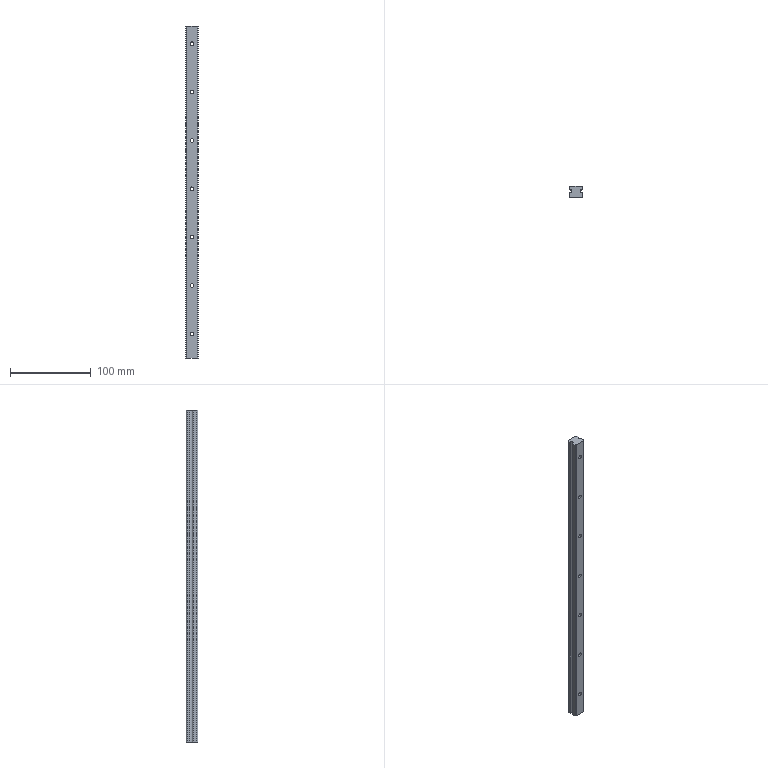Part | Creo | features CUT 8, CURVE 3, DATUM PLANE 3, COORDINATE SYSTEM 1, PATTERN 1, PROTRUSION 1 | 1 solid | 49 faces | box 14.99 x 14 x 412 mm | volume 76604 mm3 | cylinder 30 | plane 19 | commonest cylinder face diameters 4.5 x14 7.5 x14 4.48 x2
STEP:
#1=CARTESIAN_POINT('',(0.,0.,0.));
#2=DIRECTION('',(0.,0.,1.));
#3=DIRECTION('',(1.,0.,0.));
#4=AXIS2_PLACEMENT_3D('',#1,#2,#3);
#5=CARTESIAN_POINT('',(-7.49,0.995,-206.));
#6=VERTEX_POINT('',#5);
#7=CARTESIAN_POINT('',(-6.495,0.,-206.));
#8=VERTEX_POINT('',#7);
#9=CARTESIAN_POINT('',(-7.49,0.995,-206.));
#10=DIRECTION('',(0.7071,-0.7071,0.));
#11=VECTOR('',#10,1.407);
#12=LINE('',#9,#11);
#13=EDGE_CURVE('',#6,#8,#12,.T.);
#14=ORIENTED_EDGE('',*,*,#13,.T.);
#15=CARTESIAN_POINT('',(6.505,0.,-206.));
#16=VERTEX_POINT('',#15);
#17=CARTESIAN_POINT('',(-6.495,0.,-206.));
#18=DIRECTION('',(1.,0.,0.));
#19=VECTOR('',#18,13.);
#20=LINE('',#17,#19);
#21=EDGE_CURVE('',#8,#16,#20,.T.);
#22=ORIENTED_EDGE('',*,*,#21,.T.);
#23=CARTESIAN_POINT('',(7.5,0.995,-206.));
#24=VERTEX_POINT('',#23);
#25=CARTESIAN_POINT('',(6.505,0.,-206.));
#26=DIRECTION('',(0.7071,0.7071,0.));
#27=VECTOR('',#26,1.407);
#28=LINE('',#25,#27);
#29=EDGE_CURVE('',#16,#24,#28,.T.);
#30=ORIENTED_EDGE('',*,*,#29,.T.);
#31=CARTESIAN_POINT('',(7.5,5.525,-206.));
#32=VERTEX_POINT('',#31);
#33=CARTESIAN_POINT('',(7.5,0.995,-206.));
#34=DIRECTION('',(0.,1.,0.));
#35=VECTOR('',#34,4.53);
#36=LINE('',#33,#35);
#37=EDGE_CURVE('',#24,#32,#36,.T.);
#38=ORIENTED_EDGE('',*,*,#37,.T.);
#39=CARTESIAN_POINT('',(7.5,10.005,-206.));
#40=VERTEX_POINT('',#39);
#41=CARTESIAN_POINT('',(7.5,7.765,-206.));
#42=DIRECTION('',(0.,0.,-1.));
#43=DIRECTION('',(0.,-1.,0.));
#44=AXIS2_PLACEMENT_3D('',#41,#42,#43);
#45=CIRCLE('',#44,2.24);
#46=EDGE_CURVE('',#32,#40,#45,.T.);
#47=ORIENTED_EDGE('',*,*,#46,.T.);
#48=CARTESIAN_POINT('',(7.5,13.005,-206.));
#49=VERTEX_POINT('',#48);
#50=CARTESIAN_POINT('',(7.5,10.005,-206.));
#51=DIRECTION('',(0.,1.,0.));
#52=VECTOR('',#51,3.);
#53=LINE('',#50,#52);
#54=EDGE_CURVE('',#40,#49,#53,.T.);
#55=ORIENTED_EDGE('',*,*,#54,.T.);
#56=CARTESIAN_POINT('',(6.505,14.,-206.));
#57=VERTEX_POINT('',#56);
#58=CARTESIAN_POINT('',(7.5,13.005,-206.));
#59=DIRECTION('',(-0.7071,0.7071,0.));
#60=VECTOR('',#59,1.407);
#61=LINE('',#58,#60);
#62=EDGE_CURVE('',#49,#57,#61,.T.);
#63=ORIENTED_EDGE('',*,*,#62,.T.);
#64=CARTESIAN_POINT('',(-6.495,14.,-206.));
#65=VERTEX_POINT('',#64);
#66=CARTESIAN_POINT('',(6.505,14.,-206.));
#67=DIRECTION('',(-1.,0.,0.));
#68=VECTOR('',#67,13.);
#69=LINE('',#66,#68);
#70=EDGE_CURVE('',#57,#65,#69,.T.);
#71=ORIENTED_EDGE('',*,*,#70,.T.);
#72=CARTESIAN_POINT('',(-7.49,13.005,-206.));
#73=VERTEX_POINT('',#72);
#74=CARTESIAN_POINT('',(-6.495,14.,-206.));
#75=DIRECTION('',(-0.7071,-0.7071,0.));
#76=VECTOR('',#75,1.407);
#77=LINE('',#74,#76);
#78=EDGE_CURVE('',#65,#73,#77,.T.);
#79=ORIENTED_EDGE('',*,*,#78,.T.);
#80=CARTESIAN_POINT('',(-7.49,10.005,-206.));
#81=VERTEX_POINT('',#80);
#82=CARTESIAN_POINT('',(-7.49,13.005,-206.));
#83=DIRECTION('',(0.,-1.,0.));
#84=VECTOR('',#83,3.);
#85=LINE('',#82,#84);
#86=EDGE_CURVE('',#73,#81,#85,.T.);
#87=ORIENTED_EDGE('',*,*,#86,.T.);
#88=CARTESIAN_POINT('',(-7.49,5.525,-206.));
#89=VERTEX_POINT('',#88);
#90=CARTESIAN_POINT('',(-7.49,7.765,-206.));
#91=DIRECTION('',(0.,0.,-1.));
#92=DIRECTION('',(0.,1.,0.));
#93=AXIS2_PLACEMENT_3D('',#90,#91,#92);
#94=CIRCLE('',#93,2.24);
#95=EDGE_CURVE('',#81,#89,#94,.T.);
#96=ORIENTED_EDGE('',*,*,#95,.T.);
#97=CARTESIAN_POINT('',(-7.49,5.525,-206.));
#98=DIRECTION('',(0.,-1.,0.));
#99=VECTOR('',#98,4.53);
#100=LINE('',#97,#99);
#101=EDGE_CURVE('',#89,#6,#100,.T.);
#102=ORIENTED_EDGE('',*,*,#101,.T.);
#103=EDGE_LOOP('',(#14,#22,#30,#38,#47,#55,#63,#71,#79,#87,#96,#102));
#104=FACE_OUTER_BOUND('',#103,.F.);
#105=CARTESIAN_POINT('',(0.,0.,-206.));
#106=DIRECTION('',(0.,0.,1.));
#107=DIRECTION('',(1.,0.,0.));
#108=AXIS2_PLACEMENT_3D('',#105,#106,#107);
#109=PLANE('',#108);
#110=ADVANCED_FACE('',(#104),#109,.F.);
#111=ORIENTED_EDGE('',*,*,#13,.F.);
#112=CARTESIAN_POINT('',(-7.49,0.995,206.));
#113=VERTEX_POINT('',#112);
#114=CARTESIAN_POINT('',(-7.49,0.995,-206.));
#115=DIRECTION('',(0.,0.,1.));
#116=VECTOR('',#115,412.);
#117=LINE('',#114,#116);
#118=EDGE_CURVE('',#6,#113,#117,.T.);
#119=ORIENTED_EDGE('',*,*,#118,.T.);
#120=CARTESIAN_POINT('',(-6.495,0.,206.));
#121=VERTEX_POINT('',#120);
#122=CARTESIAN_POINT('',(-7.49,0.995,206.));
#123=DIRECTION('',(0.7071,-0.7071,0.));
#124=VECTOR('',#123,1.407);
#125=LINE('',#122,#124);
#126=EDGE_CURVE('',#113,#121,#125,.T.);
#127=ORIENTED_EDGE('',*,*,#126,.T.);
#128=CARTESIAN_POINT('',(-6.495,0.,-206.));
#129=DIRECTION('',(0.,0.,1.));
#130=VECTOR('',#129,412.);
#131=LINE('',#128,#130);
#132=EDGE_CURVE('',#8,#121,#131,.T.);
#133=ORIENTED_EDGE('',*,*,#132,.F.);
#134=EDGE_LOOP('',(#111,#119,#127,#133));
#135=FACE_OUTER_BOUND('',#134,.F.);
#136=CARTESIAN_POINT('',(-7.49,0.995,-206.));
#137=DIRECTION('',(-0.7071,-0.7071,0.));
#138=DIRECTION('',(0.7071,-0.7071,0.));
#139=AXIS2_PLACEMENT_3D('',#136,#137,#138);
#140=PLANE('',#139);
#141=ADVANCED_FACE('',(#135),#140,.T.);
#142=ORIENTED_EDGE('',*,*,#101,.F.);
#143=CARTESIAN_POINT('',(-7.49,5.525,206.));
#144=VERTEX_POINT('',#143);
#145=CARTESIAN_POINT('',(-7.49,5.525,-206.));
#146=DIRECTION('',(0.,0.,1.));
#147=VECTOR('',#146,412.);
#148=LINE('',#145,#147);
#149=EDGE_CURVE('',#89,#144,#148,.T.);
#150=ORIENTED_EDGE('',*,*,#149,.T.);
#151=CARTESIAN_POINT('',(-7.49,5.525,206.));
#152=DIRECTION('',(0.,-1.,0.));
#153=VECTOR('',#152,4.53);
#154=LINE('',#151,#153);
#155=EDGE_CURVE('',#144,#113,#154,.T.);
#156=ORIENTED_EDGE('',*,*,#155,.T.);
#157=ORIENTED_EDGE('',*,*,#118,.F.);
#158=EDGE_LOOP('',(#142,#150,#156,#157));
#159=FACE_OUTER_BOUND('',#158,.F.);
#160=CARTESIAN_POINT('',(-7.49,5.525,-206.));
#161=DIRECTION('',(-1.,0.,0.));
#162=DIRECTION('',(0.,-1.,0.));
#163=AXIS2_PLACEMENT_3D('',#160,#161,#162);
#164=PLANE('',#163);
#165=ADVANCED_FACE('',(#159),#164,.T.);
#166=ORIENTED_EDGE('',*,*,#95,.F.);
#167=CARTESIAN_POINT('',(-7.49,10.005,206.));
#168=VERTEX_POINT('',#167);
#169=CARTESIAN_POINT('',(-7.49,10.005,-206.));
#170=DIRECTION('',(0.,0.,1.));
#171=VECTOR('',#170,412.);
#172=LINE('',#169,#171);
#173=EDGE_CURVE('',#81,#168,#172,.T.);
#174=ORIENTED_EDGE('',*,*,#173,.T.);
#175=CARTESIAN_POINT('',(-7.49,7.765,206.));
#176=DIRECTION('',(0.,0.,-1.));
#177=DIRECTION('',(0.,1.,0.));
#178=AXIS2_PLACEMENT_3D('',#175,#176,#177);
#179=CIRCLE('',#178,2.24);
#180=EDGE_CURVE('',#168,#144,#179,.T.);
#181=ORIENTED_EDGE('',*,*,#180,.T.);
#182=ORIENTED_EDGE('',*,*,#149,.F.);
#183=EDGE_LOOP('',(#166,#174,#181,#182));
#184=FACE_OUTER_BOUND('',#183,.F.);
#185=CARTESIAN_POINT('',(-7.49,7.765,-206.));
#186=DIRECTION('',(0.,0.,1.));
#187=DIRECTION('',(1.,0.,0.));
#188=AXIS2_PLACEMENT_3D('',#185,#186,#187);
#189=CYLINDRICAL_SURFACE('',#188,2.24);
#190=ADVANCED_FACE('',(#184),#189,.F.);
#191=ORIENTED_EDGE('',*,*,#86,.F.);
#192=CARTESIAN_POINT('',(-7.49,13.005,206.));
#193=VERTEX_POINT('',#192);
#194=CARTESIAN_POINT('',(-7.49,13.005,-206.));
#195=DIRECTION('',(0.,0.,1.));
#196=VECTOR('',#195,412.);
#197=LINE('',#194,#196);
#198=EDGE_CURVE('',#73,#193,#197,.T.);
#199=ORIENTED_EDGE('',*,*,#198,.T.);
#200=CARTESIAN_POINT('',(-7.49,13.005,206.));
#201=DIRECTION('',(0.,-1.,0.));
#202=VECTOR('',#201,3.);
#203=LINE('',#200,#202);
#204=EDGE_CURVE('',#193,#168,#203,.T.);
#205=ORIENTED_EDGE('',*,*,#204,.T.);
#206=ORIENTED_EDGE('',*,*,#173,.F.);
#207=EDGE_LOOP('',(#191,#199,#205,#206));
#208=FACE_OUTER_BOUND('',#207,.F.);
#209=CARTESIAN_POINT('',(-7.49,13.005,-206.));
#210=DIRECTION('',(-1.,0.,0.));
#211=DIRECTION('',(0.,-1.,0.));
#212=AXIS2_PLACEMENT_3D('',#209,#210,#211);
#213=PLANE('',#212);
#214=ADVANCED_FACE('',(#208),#213,.T.);
#215=ORIENTED_EDGE('',*,*,#78,.F.);
#216=CARTESIAN_POINT('',(-6.495,14.,206.));
#217=VERTEX_POINT('',#216);
#218=CARTESIAN_POINT('',(-6.495,14.,-206.));
#219=DIRECTION('',(0.,0.,1.));
#220=VECTOR('',#219,412.);
#221=LINE('',#218,#220);
#222=EDGE_CURVE('',#65,#217,#221,.T.);
#223=ORIENTED_EDGE('',*,*,#222,.T.);
#224=CARTESIAN_POINT('',(-6.495,14.,206.));
#225=DIRECTION('',(-0.7071,-0.7071,0.));
#226=VECTOR('',#225,1.407);
#227=LINE('',#224,#226);
#228=EDGE_CURVE('',#217,#193,#227,.T.);
#229=ORIENTED_EDGE('',*,*,#228,.T.);
#230=ORIENTED_EDGE('',*,*,#198,.F.);
#231=EDGE_LOOP('',(#215,#223,#229,#230));
#232=FACE_OUTER_BOUND('',#231,.F.);
#233=CARTESIAN_POINT('',(-6.495,14.,-206.));
#234=DIRECTION('',(-0.7071,0.7071,0.));
#235=DIRECTION('',(-0.7071,-0.7071,0.));
#236=AXIS2_PLACEMENT_3D('',#233,#234,#235);
#237=PLANE('',#236);
#238=ADVANCED_FACE('',(#232),#237,.T.);
#239=ORIENTED_EDGE('',*,*,#70,.F.);
#240=CARTESIAN_POINT('',(6.505,14.,206.));
#241=VERTEX_POINT('',#240);
#242=CARTESIAN_POINT('',(6.505,14.,-206.));
#243=DIRECTION('',(0.,0.,1.));
#244=VECTOR('',#243,412.);
#245=LINE('',#242,#244);
#246=EDGE_CURVE('',#57,#241,#245,.T.);
#247=ORIENTED_EDGE('',*,*,#246,.T.);
#248=CARTESIAN_POINT('',(6.505,14.,206.));
#249=DIRECTION('',(-1.,0.,0.));
#250=VECTOR('',#249,13.);
#251=LINE('',#248,#250);
#252=EDGE_CURVE('',#241,#217,#251,.T.);
#253=ORIENTED_EDGE('',*,*,#252,.T.);
#254=ORIENTED_EDGE('',*,*,#222,.F.);
#255=EDGE_LOOP('',(#239,#247,#253,#254));
#256=FACE_OUTER_BOUND('',#255,.F.);
#257=CARTESIAN_POINT('',(0.,14.,-172.25));
#258=VERTEX_POINT('',#257);
#259=CARTESIAN_POINT('',(0.,14.,-179.75));
#260=VERTEX_POINT('',#259);
#261=CARTESIAN_POINT('',(0.,14.,-176.));
#262=DIRECTION('',(0.,1.,0.));
#263=DIRECTION('',(0.,0.,1.));
#264=AXIS2_PLACEMENT_3D('',#261,#262,#263);
#265=CIRCLE('',#264,3.75);
#266=EDGE_CURVE('',#258,#260,#265,.T.);
#267=ORIENTED_EDGE('',*,*,#266,.T.);
#268=CARTESIAN_POINT('',(0.,14.,-176.));
#269=DIRECTION('',(0.,1.,0.));
#270=DIRECTION('',(0.,0.,-1.));
#271=AXIS2_PLACEMENT_3D('',#268,#269,#270);
#272=CIRCLE('',#271,3.75);
#273=EDGE_CURVE('',#260,#258,#272,.T.);
#274=ORIENTED_EDGE('',*,*,#273,.T.);
#275=EDGE_LOOP('',(#267,#274));
#276=FACE_BOUND('',#275,.F.);
#277=CARTESIAN_POINT('',(0.,14.,-112.25));
#278=VERTEX_POINT('',#277);
#279=CARTESIAN_POINT('',(0.,14.,-119.75));
#280=VERTEX_POINT('',#279);
#281=CARTESIAN_POINT('',(0.,14.,-116.));
#282=DIRECTION('',(0.,1.,0.));
#283=DIRECTION('',(0.,0.,1.));
#284=AXIS2_PLACEMENT_3D('',#281,#282,#283);
#285=CIRCLE('',#284,3.75);
#286=EDGE_CURVE('',#278,#280,#285,.T.);
#287=ORIENTED_EDGE('',*,*,#286,.T.);
#288=CARTESIAN_POINT('',(0.,14.,-116.));
#289=DIRECTION('',(0.,1.,0.));
#290=DIRECTION('',(0.,0.,-1.));
#291=AXIS2_PLACEMENT_3D('',#288,#289,#290);
#292=CIRCLE('',#291,3.75);
#293=EDGE_CURVE('',#280,#278,#292,.T.);
#294=ORIENTED_EDGE('',*,*,#293,.T.);
#295=EDGE_LOOP('',(#287,#294));
#296=FACE_BOUND('',#295,.F.);
#297=CARTESIAN_POINT('',(0.,14.,-52.25));
#298=VERTEX_POINT('',#297);
#299=CARTESIAN_POINT('',(0.,14.,-59.75));
#300=VERTEX_POINT('',#299);
#301=CARTESIAN_POINT('',(0.,14.,-56.));
#302=DIRECTION('',(0.,1.,0.));
#303=DIRECTION('',(0.,0.,1.));
#304=AXIS2_PLACEMENT_3D('',#301,#302,#303);
#305=CIRCLE('',#304,3.75);
#306=EDGE_CURVE('',#298,#300,#305,.T.);
#307=ORIENTED_EDGE('',*,*,#306,.T.);
#308=CARTESIAN_POINT('',(0.,14.,-56.));
#309=DIRECTION('',(0.,1.,0.));
#310=DIRECTION('',(0.,0.,-1.));
#311=AXIS2_PLACEMENT_3D('',#308,#309,#310);
#312=CIRCLE('',#311,3.75);
#313=EDGE_CURVE('',#300,#298,#312,.T.);
#314=ORIENTED_EDGE('',*,*,#313,.T.);
#315=EDGE_LOOP('',(#307,#314));
#316=FACE_BOUND('',#315,.F.);
#317=CARTESIAN_POINT('',(0.,14.,7.75));
#318=VERTEX_POINT('',#317);
#319=CARTESIAN_POINT('',(0.,14.,0.25));
#320=VERTEX_POINT('',#319);
#321=CARTESIAN_POINT('',(0.,14.,4.));
#322=DIRECTION('',(0.,1.,0.));
#323=DIRECTION('',(0.,0.,1.));
#324=AXIS2_PLACEMENT_3D('',#321,#322,#323);
#325=CIRCLE('',#324,3.75);
#326=EDGE_CURVE('',#318,#320,#325,.T.);
#327=ORIENTED_EDGE('',*,*,#326,.T.);
#328=CARTESIAN_POINT('',(0.,14.,4.));
#329=DIRECTION('',(0.,1.,0.));
#330=DIRECTION('',(0.,0.,-1.));
#331=AXIS2_PLACEMENT_3D('',#328,#329,#330);
#332=CIRCLE('',#331,3.75);
#333=EDGE_CURVE('',#320,#318,#332,.T.);
#334=ORIENTED_EDGE('',*,*,#333,.T.);
#335=EDGE_LOOP('',(#327,#334));
#336=FACE_BOUND('',#335,.F.);
#337=CARTESIAN_POINT('',(0.,14.,67.75));
#338=VERTEX_POINT('',#337);
#339=CARTESIAN_POINT('',(0.,14.,60.25));
#340=VERTEX_POINT('',#339);
#341=CARTESIAN_POINT('',(0.,14.,64.));
#342=DIRECTION('',(0.,1.,0.));
#343=DIRECTION('',(0.,0.,1.));
#344=AXIS2_PLACEMENT_3D('',#341,#342,#343);
#345=CIRCLE('',#344,3.75);
#346=EDGE_CURVE('',#338,#340,#345,.T.);
#347=ORIENTED_EDGE('',*,*,#346,.T.);
#348=CARTESIAN_POINT('',(0.,14.,64.));
#349=DIRECTION('',(0.,1.,0.));
#350=DIRECTION('',(0.,0.,-1.));
#351=AXIS2_PLACEMENT_3D('',#348,#349,#350);
#352=CIRCLE('',#351,3.75);
#353=EDGE_CURVE('',#340,#338,#352,.T.);
#354=ORIENTED_EDGE('',*,*,#353,.T.);
#355=EDGE_LOOP('',(#347,#354));
#356=FACE_BOUND('',#355,.F.);
#357=CARTESIAN_POINT('',(0.,14.,127.75));
#358=VERTEX_POINT('',#357);
#359=CARTESIAN_POINT('',(0.,14.,120.25));
#360=VERTEX_POINT('',#359);
#361=CARTESIAN_POINT('',(0.,14.,124.));
#362=DIRECTION('',(0.,1.,0.));
#363=DIRECTION('',(0.,0.,1.));
#364=AXIS2_PLACEMENT_3D('',#361,#362,#363);
#365=CIRCLE('',#364,3.75);
#366=EDGE_CURVE('',#358,#360,#365,.T.);
#367=ORIENTED_EDGE('',*,*,#366,.T.);
#368=CARTESIAN_POINT('',(0.,14.,124.));
#369=DIRECTION('',(0.,1.,0.));
#370=DIRECTION('',(0.,0.,-1.));
#371=AXIS2_PLACEMENT_3D('',#368,#369,#370);
#372=CIRCLE('',#371,3.75);
#373=EDGE_CURVE('',#360,#358,#372,.T.);
#374=ORIENTED_EDGE('',*,*,#373,.T.);
#375=EDGE_LOOP('',(#367,#374));
#376=FACE_BOUND('',#375,.F.);
#377=CARTESIAN_POINT('',(0.,14.,187.75));
#378=VERTEX_POINT('',#377);
#379=CARTESIAN_POINT('',(0.,14.,180.25));
#380=VERTEX_POINT('',#379);
#381=CARTESIAN_POINT('',(0.,14.,184.));
#382=DIRECTION('',(0.,1.,0.));
#383=DIRECTION('',(0.,0.,1.));
#384=AXIS2_PLACEMENT_3D('',#381,#382,#383);
#385=CIRCLE('',#384,3.75);
#386=EDGE_CURVE('',#378,#380,#385,.T.);
#387=ORIENTED_EDGE('',*,*,#386,.T.);
#388=CARTESIAN_POINT('',(0.,14.,184.));
#389=DIRECTION('',(0.,1.,0.));
#390=DIRECTION('',(0.,0.,-1.));
#391=AXIS2_PLACEMENT_3D('',#388,#389,#390);
#392=CIRCLE('',#391,3.75);
#393=EDGE_CURVE('',#380,#378,#392,.T.);
#394=ORIENTED_EDGE('',*,*,#393,.T.);
#395=EDGE_LOOP('',(#387,#394));
#396=FACE_BOUND('',#395,.F.);
#397=CARTESIAN_POINT('',(6.505,14.,-206.));
#398=DIRECTION('',(0.,1.,0.));
#399=DIRECTION('',(-1.,0.,0.));
#400=AXIS2_PLACEMENT_3D('',#397,#398,#399);
#401=PLANE('',#400);
#402=ADVANCED_FACE('',(#256,#276,#296,#316,#336,#356,#376,#396),#401,.T.);
#403=ORIENTED_EDGE('',*,*,#62,.F.);
#404=CARTESIAN_POINT('',(7.5,13.005,206.));
#405=VERTEX_POINT('',#404);
#406=CARTESIAN_POINT('',(7.5,13.005,-206.));
#407=DIRECTION('',(0.,0.,1.));
#408=VECTOR('',#407,412.);
#409=LINE('',#406,#408);
#410=EDGE_CURVE('',#49,#405,#409,.T.);
#411=ORIENTED_EDGE('',*,*,#410,.T.);
#412=CARTESIAN_POINT('',(7.5,13.005,206.));
#413=DIRECTION('',(-0.7071,0.7071,0.));
#414=VECTOR('',#413,1.407);
#415=LINE('',#412,#414);
#416=EDGE_CURVE('',#405,#241,#415,.T.);
#417=ORIENTED_EDGE('',*,*,#416,.T.);
#418=ORIENTED_EDGE('',*,*,#246,.F.);
#419=EDGE_LOOP('',(#403,#411,#417,#418));
#420=FACE_OUTER_BOUND('',#419,.F.);
#421=CARTESIAN_POINT('',(7.5,13.005,-206.));
#422=DIRECTION('',(0.7071,0.7071,0.));
#423=DIRECTION('',(-0.7071,0.7071,0.));
#424=AXIS2_PLACEMENT_3D('',#421,#422,#423);
#425=PLANE('',#424);
#426=ADVANCED_FACE('',(#420),#425,.T.);
#427=ORIENTED_EDGE('',*,*,#54,.F.);
#428=CARTESIAN_POINT('',(7.5,10.005,206.));
#429=VERTEX_POINT('',#428);
#430=CARTESIAN_POINT('',(7.5,10.005,-206.));
#431=DIRECTION('',(0.,0.,1.));
#432=VECTOR('',#431,412.);
#433=LINE('',#430,#432);
#434=EDGE_CURVE('',#40,#429,#433,.T.);
#435=ORIENTED_EDGE('',*,*,#434,.T.);
#436=CARTESIAN_POINT('',(7.5,10.005,206.));
#437=DIRECTION('',(0.,1.,0.));
#438=VECTOR('',#437,3.);
#439=LINE('',#436,#438);
#440=EDGE_CURVE('',#429,#405,#439,.T.);
#441=ORIENTED_EDGE('',*,*,#440,.T.);
#442=ORIENTED_EDGE('',*,*,#410,.F.);
#443=EDGE_LOOP('',(#427,#435,#441,#442));
#444=FACE_OUTER_BOUND('',#443,.F.);
#445=CARTESIAN_POINT('',(7.5,10.005,-206.));
#446=DIRECTION('',(1.,0.,0.));
#447=DIRECTION('',(0.,1.,0.));
#448=AXIS2_PLACEMENT_3D('',#445,#446,#447);
#449=PLANE('',#448);
#450=ADVANCED_FACE('',(#444),#449,.T.);
#451=ORIENTED_EDGE('',*,*,#46,.F.);
#452=CARTESIAN_POINT('',(7.5,5.525,206.));
#453=VERTEX_POINT('',#452);
#454=CARTESIAN_POINT('',(7.5,5.525,-206.));
#455=DIRECTION('',(0.,0.,1.));
#456=VECTOR('',#455,412.);
#457=LINE('',#454,#456);
#458=EDGE_CURVE('',#32,#453,#457,.T.);
#459=ORIENTED_EDGE('',*,*,#458,.T.);
#460=CARTESIAN_POINT('',(7.5,7.765,206.));
#461=DIRECTION('',(0.,0.,-1.));
#462=DIRECTION('',(0.,-1.,0.));
#463=AXIS2_PLACEMENT_3D('',#460,#461,#462);
#464=CIRCLE('',#463,2.24);
#465=EDGE_CURVE('',#453,#429,#464,.T.);
#466=ORIENTED_EDGE('',*,*,#465,.T.);
#467=ORIENTED_EDGE('',*,*,#434,.F.);
#468=EDGE_LOOP('',(#451,#459,#466,#467));
#469=FACE_OUTER_BOUND('',#468,.F.);
#470=CARTESIAN_POINT('',(7.5,7.765,-206.));
#471=DIRECTION('',(0.,0.,1.));
#472=DIRECTION('',(1.,0.,0.));
#473=AXIS2_PLACEMENT_3D('',#470,#471,#472);
#474=CYLINDRICAL_SURFACE('',#473,2.24);
#475=ADVANCED_FACE('',(#469),#474,.F.);
#476=ORIENTED_EDGE('',*,*,#37,.F.);
#477=CARTESIAN_POINT('',(7.5,0.995,206.));
#478=VERTEX_POINT('',#477);
#479=CARTESIAN_POINT('',(7.5,0.995,-206.));
#480=DIRECTION('',(0.,0.,1.));
#481=VECTOR('',#480,412.);
#482=LINE('',#479,#481);
#483=EDGE_CURVE('',#24,#478,#482,.T.);
#484=ORIENTED_EDGE('',*,*,#483,.T.);
#485=CARTESIAN_POINT('',(7.5,0.995,206.));
#486=DIRECTION('',(0.,1.,0.));
#487=VECTOR('',#486,4.53);
#488=LINE('',#485,#487);
#489=EDGE_CURVE('',#478,#453,#488,.T.);
#490=ORIENTED_EDGE('',*,*,#489,.T.);
#491=ORIENTED_EDGE('',*,*,#458,.F.);
#492=EDGE_LOOP('',(#476,#484,#490,#491));
#493=FACE_OUTER_BOUND('',#492,.F.);
#494=CARTESIAN_POINT('',(7.5,0.995,-206.));
#495=DIRECTION('',(1.,0.,0.));
#496=DIRECTION('',(0.,1.,0.));
#497=AXIS2_PLACEMENT_3D('',#494,#495,#496);
#498=PLANE('',#497);
#499=ADVANCED_FACE('',(#493),#498,.T.);
#500=ORIENTED_EDGE('',*,*,#29,.F.);
#501=CARTESIAN_POINT('',(6.505,0.,206.));
#502=VERTEX_POINT('',#501);
#503=CARTESIAN_POINT('',(6.505,0.,-206.));
#504=DIRECTION('',(0.,0.,1.));
#505=VECTOR('',#504,412.);
#506=LINE('',#503,#505);
#507=EDGE_CURVE('',#16,#502,#506,.T.);
#508=ORIENTED_EDGE('',*,*,#507,.T.);
#509=CARTESIAN_POINT('',(6.505,0.,206.));
#510=DIRECTION('',(0.7071,0.7071,0.));
#511=VECTOR('',#510,1.407);
#512=LINE('',#509,#511);
#513=EDGE_CURVE('',#502,#478,#512,.T.);
#514=ORIENTED_EDGE('',*,*,#513,.T.);
#515=ORIENTED_EDGE('',*,*,#483,.F.);
#516=EDGE_LOOP('',(#500,#508,#514,#515));
#517=FACE_OUTER_BOUND('',#516,.F.);
#518=CARTESIAN_POINT('',(6.505,0.,-206.));
#519=DIRECTION('',(0.7071,-0.7071,0.));
#520=DIRECTION('',(0.7071,0.7071,0.));
#521=AXIS2_PLACEMENT_3D('',#518,#519,#520);
#522=PLANE('',#521);
#523=ADVANCED_FACE('',(#517),#522,.T.);
#524=ORIENTED_EDGE('',*,*,#21,.F.);
#525=ORIENTED_EDGE('',*,*,#132,.T.);
#526=CARTESIAN_POINT('',(-6.495,0.,206.));
#527=DIRECTION('',(1.,0.,0.));
#528=VECTOR('',#527,13.);
#529=LINE('',#526,#528);
#530=EDGE_CURVE('',#121,#502,#529,.T.);
#531=ORIENTED_EDGE('',*,*,#530,.T.);
#532=ORIENTED_EDGE('',*,*,#507,.F.);
#533=EDGE_LOOP('',(#524,#525,#531,#532));
#534=FACE_OUTER_BOUND('',#533,.F.);
#535=CARTESIAN_POINT('',(0.,0.,-173.75));
#536=VERTEX_POINT('',#535);
#537=CARTESIAN_POINT('',(0.,0.,-178.25));
#538=VERTEX_POINT('',#537);
#539=CARTESIAN_POINT('',(0.,0.,-176.));
#540=DIRECTION('',(0.,1.,0.));
#541=DIRECTION('',(0.,0.,1.));
#542=AXIS2_PLACEMENT_3D('',#539,#540,#541);
#543=CIRCLE('',#542,2.25);
#544=EDGE_CURVE('',#536,#538,#543,.T.);
#545=ORIENTED_EDGE('',*,*,#544,.F.);
#546=CARTESIAN_POINT('',(0.,0.,-176.));
#547=DIRECTION('',(0.,1.,0.));
#548=DIRECTION('',(0.,0.,-1.));
#549=AXIS2_PLACEMENT_3D('',#546,#547,#548);
#550=CIRCLE('',#549,2.25);
#551=EDGE_CURVE('',#538,#536,#550,.T.);
#552=ORIENTED_EDGE('',*,*,#551,.F.);
#553=EDGE_LOOP('',(#545,#552));
#554=FACE_BOUND('',#553,.F.);
#555=CARTESIAN_POINT('',(0.,0.,-113.75));
#556=VERTEX_POINT('',#555);
#557=CARTESIAN_POINT('',(0.,0.,-118.25));
#558=VERTEX_POINT('',#557);
#559=CARTESIAN_POINT('',(0.,0.,-116.));
#560=DIRECTION('',(0.,1.,0.));
#561=DIRECTION('',(0.,0.,1.));
#562=AXIS2_PLACEMENT_3D('',#559,#560,#561);
#563=CIRCLE('',#562,2.25);
#564=EDGE_CURVE('',#556,#558,#563,.T.);
#565=ORIENTED_EDGE('',*,*,#564,.F.);
#566=CARTESIAN_POINT('',(0.,0.,-116.));
#567=DIRECTION('',(0.,1.,0.));
#568=DIRECTION('',(0.,0.,-1.));
#569=AXIS2_PLACEMENT_3D('',#566,#567,#568);
#570=CIRCLE('',#569,2.25);
#571=EDGE_CURVE('',#558,#556,#570,.T.);
#572=ORIENTED_EDGE('',*,*,#571,.F.);
#573=EDGE_LOOP('',(#565,#572));
#574=FACE_BOUND('',#573,.F.);
#575=CARTESIAN_POINT('',(0.,0.,-53.75));
#576=VERTEX_POINT('',#575);
#577=CARTESIAN_POINT('',(0.,0.,-58.25));
#578=VERTEX_POINT('',#577);
#579=CARTESIAN_POINT('',(0.,0.,-56.));
#580=DIRECTION('',(0.,1.,0.));
#581=DIRECTION('',(0.,0.,1.));
#582=AXIS2_PLACEMENT_3D('',#579,#580,#581);
#583=CIRCLE('',#582,2.25);
#584=EDGE_CURVE('',#576,#578,#583,.T.);
#585=ORIENTED_EDGE('',*,*,#584,.F.);
#586=CARTESIAN_POINT('',(0.,0.,-56.));
#587=DIRECTION('',(0.,1.,0.));
#588=DIRECTION('',(0.,0.,-1.));
#589=AXIS2_PLACEMENT_3D('',#586,#587,#588);
#590=CIRCLE('',#589,2.25);
#591=EDGE_CURVE('',#578,#576,#590,.T.);
#592=ORIENTED_EDGE('',*,*,#591,.F.);
#593=EDGE_LOOP('',(#585,#592));
#594=FACE_BOUND('',#593,.F.);
#595=CARTESIAN_POINT('',(0.,0.,6.25));
#596=VERTEX_POINT('',#595);
#597=CARTESIAN_POINT('',(0.,0.,1.75));
#598=VERTEX_POINT('',#597);
#599=CARTESIAN_POINT('',(0.,0.,4.));
#600=DIRECTION('',(0.,1.,0.));
#601=DIRECTION('',(0.,0.,1.));
#602=AXIS2_PLACEMENT_3D('',#599,#600,#601);
#603=CIRCLE('',#602,2.25);
#604=EDGE_CURVE('',#596,#598,#603,.T.);
#605=ORIENTED_EDGE('',*,*,#604,.F.);
#606=CARTESIAN_POINT('',(0.,0.,4.));
#607=DIRECTION('',(0.,1.,0.));
#608=DIRECTION('',(0.,0.,-1.));
#609=AXIS2_PLACEMENT_3D('',#606,#607,#608);
#610=CIRCLE('',#609,2.25);
#611=EDGE_CURVE('',#598,#596,#610,.T.);
#612=ORIENTED_EDGE('',*,*,#611,.F.);
#613=EDGE_LOOP('',(#605,#612));
#614=FACE_BOUND('',#613,.F.);
#615=CARTESIAN_POINT('',(0.,0.,66.25));
#616=VERTEX_POINT('',#615);
#617=CARTESIAN_POINT('',(0.,0.,61.75));
#618=VERTEX_POINT('',#617);
#619=CARTESIAN_POINT('',(0.,0.,64.));
#620=DIRECTION('',(0.,1.,0.));
#621=DIRECTION('',(0.,0.,1.));
#622=AXIS2_PLACEMENT_3D('',#619,#620,#621);
#623=CIRCLE('',#622,2.25);
#624=EDGE_CURVE('',#616,#618,#623,.T.);
#625=ORIENTED_EDGE('',*,*,#624,.F.);
#626=CARTESIAN_POINT('',(0.,0.,64.));
#627=DIRECTION('',(0.,1.,0.));
#628=DIRECTION('',(0.,0.,-1.));
#629=AXIS2_PLACEMENT_3D('',#626,#627,#628);
#630=CIRCLE('',#629,2.25);
#631=EDGE_CURVE('',#618,#616,#630,.T.);
#632=ORIENTED_EDGE('',*,*,#631,.F.);
#633=EDGE_LOOP('',(#625,#632));
#634=FACE_BOUND('',#633,.F.);
#635=CARTESIAN_POINT('',(0.,0.,126.25));
#636=VERTEX_POINT('',#635);
#637=CARTESIAN_POINT('',(0.,0.,121.75));
#638=VERTEX_POINT('',#637);
#639=CARTESIAN_POINT('',(0.,0.,124.));
#640=DIRECTION('',(0.,1.,0.));
#641=DIRECTION('',(0.,0.,1.));
#642=AXIS2_PLACEMENT_3D('',#639,#640,#641);
#643=CIRCLE('',#642,2.25);
#644=EDGE_CURVE('',#636,#638,#643,.T.);
#645=ORIENTED_EDGE('',*,*,#644,.F.);
#646=CARTESIAN_POINT('',(0.,0.,124.));
#647=DIRECTION('',(0.,1.,0.));
#648=DIRECTION('',(0.,0.,-1.));
#649=AXIS2_PLACEMENT_3D('',#646,#647,#648);
#650=CIRCLE('',#649,2.25);
#651=EDGE_CURVE('',#638,#636,#650,.T.);
#652=ORIENTED_EDGE('',*,*,#651,.F.);
#653=EDGE_LOOP('',(#645,#652));
#654=FACE_BOUND('',#653,.F.);
#655=CARTESIAN_POINT('',(0.,0.,186.25));
#656=VERTEX_POINT('',#655);
#657=CARTESIAN_POINT('',(0.,0.,181.75));
#658=VERTEX_POINT('',#657);
#659=CARTESIAN_POINT('',(0.,0.,184.));
#660=DIRECTION('',(0.,1.,0.));
#661=DIRECTION('',(0.,0.,1.));
#662=AXIS2_PLACEMENT_3D('',#659,#660,#661);
#663=CIRCLE('',#662,2.25);
#664=EDGE_CURVE('',#656,#658,#663,.T.);
#665=ORIENTED_EDGE('',*,*,#664,.F.);
#666=CARTESIAN_POINT('',(0.,0.,184.));
#667=DIRECTION('',(0.,1.,0.));
#668=DIRECTION('',(0.,0.,-1.));
#669=AXIS2_PLACEMENT_3D('',#666,#667,#668);
#670=CIRCLE('',#669,2.25);
#671=EDGE_CURVE('',#658,#656,#670,.T.);
#672=ORIENTED_EDGE('',*,*,#671,.F.);
#673=EDGE_LOOP('',(#665,#672));
#674=FACE_BOUND('',#673,.F.);
#675=CARTESIAN_POINT('',(-6.495,0.,-206.));
#676=DIRECTION('',(0.,-1.,0.));
#677=DIRECTION('',(1.,0.,0.));
#678=AXIS2_PLACEMENT_3D('',#675,#676,#677);
#679=PLANE('',#678);
#680=ADVANCED_FACE('',(#534,#554,#574,#594,#614,#634,#654,#674),#679,.T.);
#681=ORIENTED_EDGE('',*,*,#126,.F.);
#682=ORIENTED_EDGE('',*,*,#155,.F.);
#683=ORIENTED_EDGE('',*,*,#180,.F.);
#684=ORIENTED_EDGE('',*,*,#204,.F.);
#685=ORIENTED_EDGE('',*,*,#228,.F.);
#686=ORIENTED_EDGE('',*,*,#252,.F.);
#687=ORIENTED_EDGE('',*,*,#416,.F.);
#688=ORIENTED_EDGE('',*,*,#440,.F.);
#689=ORIENTED_EDGE('',*,*,#465,.F.);
#690=ORIENTED_EDGE('',*,*,#489,.F.);
#691=ORIENTED_EDGE('',*,*,#513,.F.);
#692=ORIENTED_EDGE('',*,*,#530,.F.);
#693=EDGE_LOOP('',(#681,#682,#683,#684,#685,#686,#687,#688,#689,#690,#691,#692));
#694=FACE_OUTER_BOUND('',#693,.F.);
#695=CARTESIAN_POINT('',(0.,0.,206.));
#696=DIRECTION('',(0.,0.,1.));
#697=DIRECTION('',(1.,0.,0.));
#698=AXIS2_PLACEMENT_3D('',#695,#696,#697);
#699=PLANE('',#698);
#700=ADVANCED_FACE('',(#694),#699,.T.);
#701=CARTESIAN_POINT('',(0.,9.,-173.75));
#702=VERTEX_POINT('',#701);
#703=CARTESIAN_POINT('',(0.,9.,-178.25));
#704=VERTEX_POINT('',#703);
#705=CARTESIAN_POINT('',(0.,9.,-176.));
#706=DIRECTION('',(0.,1.,0.));
#707=DIRECTION('',(0.,0.,1.));
#708=AXIS2_PLACEMENT_3D('',#705,#706,#707);
#709=CIRCLE('',#708,2.25);
#710=EDGE_CURVE('',#702,#704,#709,.T.);
#711=ORIENTED_EDGE('',*,*,#710,.F.);
#712=CARTESIAN_POINT('',(0.,9.,-173.75));
#713=DIRECTION('',(0.,-1.,0.));
#714=VECTOR('',#713,9.);
#715=LINE('',#712,#714);
#716=EDGE_CURVE('',#702,#536,#715,.T.);
#717=ORIENTED_EDGE('',*,*,#716,.T.);
#718=ORIENTED_EDGE('',*,*,#544,.T.);
#719=CARTESIAN_POINT('',(0.,9.,-178.25));
#720=DIRECTION('',(0.,-1.,0.));
#721=VECTOR('',#720,9.);
#722=LINE('',#719,#721);
#723=EDGE_CURVE('',#704,#538,#722,.T.);
#724=ORIENTED_EDGE('',*,*,#723,.F.);
#725=EDGE_LOOP('',(#711,#717,#718,#724));
#726=FACE_OUTER_BOUND('',#725,.F.);
#727=CARTESIAN_POINT('',(0.,14.,-176.));
#728=DIRECTION('',(0.,1.,0.));
#729=DIRECTION('',(0.,0.,1.));
#730=AXIS2_PLACEMENT_3D('',#727,#728,#729);
#731=CYLINDRICAL_SURFACE('',#730,2.25);
#732=ADVANCED_FACE('',(#726),#731,.F.);
#733=CARTESIAN_POINT('',(0.,9.,-172.25));
#734=VERTEX_POINT('',#733);
#735=CARTESIAN_POINT('',(0.,9.,-179.75));
#736=VERTEX_POINT('',#735);
#737=CARTESIAN_POINT('',(0.,9.,-176.));
#738=DIRECTION('',(0.,1.,0.));
#739=DIRECTION('',(0.,0.,1.));
#740=AXIS2_PLACEMENT_3D('',#737,#738,#739);
#741=CIRCLE('',#740,3.75);
#742=EDGE_CURVE('',#734,#736,#741,.T.);
#743=ORIENTED_EDGE('',*,*,#742,.F.);
#744=CARTESIAN_POINT('',(0.,9.,-176.));
#745=DIRECTION('',(0.,1.,0.));
#746=DIRECTION('',(0.,0.,-1.));
#747=AXIS2_PLACEMENT_3D('',#744,#745,#746);
#748=CIRCLE('',#747,3.75);
#749=EDGE_CURVE('',#736,#734,#748,.T.);
#750=ORIENTED_EDGE('',*,*,#749,.F.);
#751=EDGE_LOOP('',(#743,#750));
#752=FACE_OUTER_BOUND('',#751,.F.);
#753=ORIENTED_EDGE('',*,*,#710,.T.);
#754=CARTESIAN_POINT('',(0.,9.,-176.));
#755=DIRECTION('',(0.,1.,0.));
#756=DIRECTION('',(0.,0.,-1.));
#757=AXIS2_PLACEMENT_3D('',#754,#755,#756);
#758=CIRCLE('',#757,2.25);
#759=EDGE_CURVE('',#704,#702,#758,.T.);
#760=ORIENTED_EDGE('',*,*,#759,.T.);
#761=EDGE_LOOP('',(#753,#760));
#762=FACE_BOUND('',#761,.F.);
#763=CARTESIAN_POINT('',(0.,9.,-206.));
#764=DIRECTION('',(0.,1.,0.));
#765=DIRECTION('',(0.,0.,1.));
#766=AXIS2_PLACEMENT_3D('',#763,#764,#765);
#767=PLANE('',#766);
#768=ADVANCED_FACE('',(#752,#762),#767,.T.);
#769=CARTESIAN_POINT('',(0.,9.,-112.25));
#770=VERTEX_POINT('',#769);
#771=CARTESIAN_POINT('',(0.,9.,-119.75));
#772=VERTEX_POINT('',#771);
#773=CARTESIAN_POINT('',(0.,9.,-116.));
#774=DIRECTION('',(0.,1.,0.));
#775=DIRECTION('',(0.,0.,1.));
#776=AXIS2_PLACEMENT_3D('',#773,#774,#775);
#777=CIRCLE('',#776,3.75);
#778=EDGE_CURVE('',#770,#772,#777,.T.);
#779=ORIENTED_EDGE('',*,*,#778,.F.);
#780=CARTESIAN_POINT('',(0.,9.,-116.));
#781=DIRECTION('',(0.,1.,0.));
#782=DIRECTION('',(0.,0.,-1.));
#783=AXIS2_PLACEMENT_3D('',#780,#781,#782);
#784=CIRCLE('',#783,3.75);
#785=EDGE_CURVE('',#772,#770,#784,.T.);
#786=ORIENTED_EDGE('',*,*,#785,.F.);
#787=EDGE_LOOP('',(#779,#786));
#788=FACE_OUTER_BOUND('',#787,.F.);
#789=CARTESIAN_POINT('',(0.,9.,-113.75));
#790=VERTEX_POINT('',#789);
#791=CARTESIAN_POINT('',(0.,9.,-118.25));
#792=VERTEX_POINT('',#791);
#793=CARTESIAN_POINT('',(0.,9.,-116.));
#794=DIRECTION('',(0.,1.,0.));
#795=DIRECTION('',(0.,0.,1.));
#796=AXIS2_PLACEMENT_3D('',#793,#794,#795);
#797=CIRCLE('',#796,2.25);
#798=EDGE_CURVE('',#790,#792,#797,.T.);
#799=ORIENTED_EDGE('',*,*,#798,.T.);
#800=CARTESIAN_POINT('',(0.,9.,-116.));
#801=DIRECTION('',(0.,1.,0.));
#802=DIRECTION('',(0.,0.,-1.));
#803=AXIS2_PLACEMENT_3D('',#800,#801,#802);
#804=CIRCLE('',#803,2.25);
#805=EDGE_CURVE('',#792,#790,#804,.T.);
#806=ORIENTED_EDGE('',*,*,#805,.T.);
#807=EDGE_LOOP('',(#799,#806));
#808=FACE_BOUND('',#807,.F.);
#809=CARTESIAN_POINT('',(0.,9.,-206.));
#810=DIRECTION('',(0.,1.,0.));
#811=DIRECTION('',(0.,0.,1.));
#812=AXIS2_PLACEMENT_3D('',#809,#810,#811);
#813=PLANE('',#812);
#814=ADVANCED_FACE('',(#788,#808),#813,.T.);
#815=CARTESIAN_POINT('',(0.,9.,-52.25));
#816=VERTEX_POINT('',#815);
#817=CARTESIAN_POINT('',(0.,9.,-59.75));
#818=VERTEX_POINT('',#817);
#819=CARTESIAN_POINT('',(0.,9.,-56.));
#820=DIRECTION('',(0.,1.,0.));
#821=DIRECTION('',(0.,0.,1.));
#822=AXIS2_PLACEMENT_3D('',#819,#820,#821);
#823=CIRCLE('',#822,3.75);
#824=EDGE_CURVE('',#816,#818,#823,.T.);
#825=ORIENTED_EDGE('',*,*,#824,.F.);
#826=CARTESIAN_POINT('',(0.,9.,-56.));
#827=DIRECTION('',(0.,1.,0.));
#828=DIRECTION('',(0.,0.,-1.));
#829=AXIS2_PLACEMENT_3D('',#826,#827,#828);
#830=CIRCLE('',#829,3.75);
#831=EDGE_CURVE('',#818,#816,#830,.T.);
#832=ORIENTED_EDGE('',*,*,#831,.F.);
#833=EDGE_LOOP('',(#825,#832));
#834=FACE_OUTER_BOUND('',#833,.F.);
#835=CARTESIAN_POINT('',(0.,9.,-53.75));
#836=VERTEX_POINT('',#835);
#837=CARTESIAN_POINT('',(0.,9.,-58.25));
#838=VERTEX_POINT('',#837);
#839=CARTESIAN_POINT('',(0.,9.,-56.));
#840=DIRECTION('',(0.,1.,0.));
#841=DIRECTION('',(0.,0.,1.));
#842=AXIS2_PLACEMENT_3D('',#839,#840,#841);
#843=CIRCLE('',#842,2.25);
#844=EDGE_CURVE('',#836,#838,#843,.T.);
#845=ORIENTED_EDGE('',*,*,#844,.T.);
#846=CARTESIAN_POINT('',(0.,9.,-56.));
#847=DIRECTION('',(0.,1.,0.));
#848=DIRECTION('',(0.,0.,-1.));
#849=AXIS2_PLACEMENT_3D('',#846,#847,#848);
#850=CIRCLE('',#849,2.25);
#851=EDGE_CURVE('',#838,#836,#850,.T.);
#852=ORIENTED_EDGE('',*,*,#851,.T.);
#853=EDGE_LOOP('',(#845,#852));
#854=FACE_BOUND('',#853,.F.);
#855=CARTESIAN_POINT('',(0.,9.,-206.));
#856=DIRECTION('',(0.,1.,0.));
#857=DIRECTION('',(0.,0.,1.));
#858=AXIS2_PLACEMENT_3D('',#855,#856,#857);
#859=PLANE('',#858);
#860=ADVANCED_FACE('',(#834,#854),#859,.T.);
#861=CARTESIAN_POINT('',(0.,9.,7.75));
#862=VERTEX_POINT('',#861);
#863=CARTESIAN_POINT('',(0.,9.,0.25));
#864=VERTEX_POINT('',#863);
#865=CARTESIAN_POINT('',(0.,9.,4.));
#866=DIRECTION('',(0.,1.,0.));
#867=DIRECTION('',(0.,0.,1.));
#868=AXIS2_PLACEMENT_3D('',#865,#866,#867);
#869=CIRCLE('',#868,3.75);
#870=EDGE_CURVE('',#862,#864,#869,.T.);
#871=ORIENTED_EDGE('',*,*,#870,.F.);
#872=CARTESIAN_POINT('',(0.,9.,4.));
#873=DIRECTION('',(0.,1.,0.));
#874=DIRECTION('',(0.,0.,-1.));
#875=AXIS2_PLACEMENT_3D('',#872,#873,#874);
#876=CIRCLE('',#875,3.75);
#877=EDGE_CURVE('',#864,#862,#876,.T.);
#878=ORIENTED_EDGE('',*,*,#877,.F.);
#879=EDGE_LOOP('',(#871,#878));
#880=FACE_OUTER_BOUND('',#879,.F.);
#881=CARTESIAN_POINT('',(0.,9.,6.25));
#882=VERTEX_POINT('',#881);
#883=CARTESIAN_POINT('',(0.,9.,1.75));
#884=VERTEX_POINT('',#883);
#885=CARTESIAN_POINT('',(0.,9.,4.));
#886=DIRECTION('',(0.,1.,0.));
#887=DIRECTION('',(0.,0.,1.));
#888=AXIS2_PLACEMENT_3D('',#885,#886,#887);
#889=CIRCLE('',#888,2.25);
#890=EDGE_CURVE('',#882,#884,#889,.T.);
#891=ORIENTED_EDGE('',*,*,#890,.T.);
#892=CARTESIAN_POINT('',(0.,9.,4.));
#893=DIRECTION('',(0.,1.,0.));
#894=DIRECTION('',(0.,0.,-1.));
#895=AXIS2_PLACEMENT_3D('',#892,#893,#894);
#896=CIRCLE('',#895,2.25);
#897=EDGE_CURVE('',#884,#882,#896,.T.);
#898=ORIENTED_EDGE('',*,*,#897,.T.);
#899=EDGE_LOOP('',(#891,#898));
#900=FACE_BOUND('',#899,.F.);
#901=CARTESIAN_POINT('',(0.,9.,-206.));
#902=DIRECTION('',(0.,1.,0.));
#903=DIRECTION('',(0.,0.,1.));
#904=AXIS2_PLACEMENT_3D('',#901,#902,#903);
#905=PLANE('',#904);
#906=ADVANCED_FACE('',(#880,#900),#905,.T.);
#907=CARTESIAN_POINT('',(0.,9.,67.75));
#908=VERTEX_POINT('',#907);
#909=CARTESIAN_POINT('',(0.,9.,60.25));
#910=VERTEX_POINT('',#909);
#911=CARTESIAN_POINT('',(0.,9.,64.));
#912=DIRECTION('',(0.,1.,0.));
#913=DIRECTION('',(0.,0.,1.));
#914=AXIS2_PLACEMENT_3D('',#911,#912,#913);
#915=CIRCLE('',#914,3.75);
#916=EDGE_CURVE('',#908,#910,#915,.T.);
#917=ORIENTED_EDGE('',*,*,#916,.F.);
#918=CARTESIAN_POINT('',(0.,9.,64.));
#919=DIRECTION('',(0.,1.,0.));
#920=DIRECTION('',(0.,0.,-1.));
#921=AXIS2_PLACEMENT_3D('',#918,#919,#920);
#922=CIRCLE('',#921,3.75);
#923=EDGE_CURVE('',#910,#908,#922,.T.);
#924=ORIENTED_EDGE('',*,*,#923,.F.);
#925=EDGE_LOOP('',(#917,#924));
#926=FACE_OUTER_BOUND('',#925,.F.);
#927=CARTESIAN_POINT('',(0.,9.,66.25));
#928=VERTEX_POINT('',#927);
#929=CARTESIAN_POINT('',(0.,9.,61.75));
#930=VERTEX_POINT('',#929);
#931=CARTESIAN_POINT('',(0.,9.,64.));
#932=DIRECTION('',(0.,1.,0.));
#933=DIRECTION('',(0.,0.,1.));
#934=AXIS2_PLACEMENT_3D('',#931,#932,#933);
#935=CIRCLE('',#934,2.25);
#936=EDGE_CURVE('',#928,#930,#935,.T.);
#937=ORIENTED_EDGE('',*,*,#936,.T.);
#938=CARTESIAN_POINT('',(0.,9.,64.));
#939=DIRECTION('',(0.,1.,0.));
#940=DIRECTION('',(0.,0.,-1.));
#941=AXIS2_PLACEMENT_3D('',#938,#939,#940);
#942=CIRCLE('',#941,2.25);
#943=EDGE_CURVE('',#930,#928,#942,.T.);
#944=ORIENTED_EDGE('',*,*,#943,.T.);
#945=EDGE_LOOP('',(#937,#944));
#946=FACE_BOUND('',#945,.F.);
#947=CARTESIAN_POINT('',(0.,9.,-206.));
#948=DIRECTION('',(0.,1.,0.));
#949=DIRECTION('',(0.,0.,1.));
#950=AXIS2_PLACEMENT_3D('',#947,#948,#949);
#951=PLANE('',#950);
#952=ADVANCED_FACE('',(#926,#946),#951,.T.);
#953=CARTESIAN_POINT('',(0.,9.,127.75));
#954=VERTEX_POINT('',#953);
#955=CARTESIAN_POINT('',(0.,9.,120.25));
#956=VERTEX_POINT('',#955);
#957=CARTESIAN_POINT('',(0.,9.,124.));
#958=DIRECTION('',(0.,1.,0.));
#959=DIRECTION('',(0.,0.,1.));
#960=AXIS2_PLACEMENT_3D('',#957,#958,#959);
#961=CIRCLE('',#960,3.75);
#962=EDGE_CURVE('',#954,#956,#961,.T.);
#963=ORIENTED_EDGE('',*,*,#962,.F.);
#964=CARTESIAN_POINT('',(0.,9.,124.));
#965=DIRECTION('',(0.,1.,0.));
#966=DIRECTION('',(0.,0.,-1.));
#967=AXIS2_PLACEMENT_3D('',#964,#965,#966);
#968=CIRCLE('',#967,3.75);
#969=EDGE_CURVE('',#956,#954,#968,.T.);
#970=ORIENTED_EDGE('',*,*,#969,.F.);
#971=EDGE_LOOP('',(#963,#970));
#972=FACE_OUTER_BOUND('',#971,.F.);
#973=CARTESIAN_POINT('',(0.,9.,126.25));
#974=VERTEX_POINT('',#973);
#975=CARTESIAN_POINT('',(0.,9.,121.75));
#976=VERTEX_POINT('',#975);
#977=CARTESIAN_POINT('',(0.,9.,124.));
#978=DIRECTION('',(0.,1.,0.));
#979=DIRECTION('',(0.,0.,1.));
#980=AXIS2_PLACEMENT_3D('',#977,#978,#979);
#981=CIRCLE('',#980,2.25);
#982=EDGE_CURVE('',#974,#976,#981,.T.);
#983=ORIENTED_EDGE('',*,*,#982,.T.);
#984=CARTESIAN_POINT('',(0.,9.,124.));
#985=DIRECTION('',(0.,1.,0.));
#986=DIRECTION('',(0.,0.,-1.));
#987=AXIS2_PLACEMENT_3D('',#984,#985,#986);
#988=CIRCLE('',#987,2.25);
#989=EDGE_CURVE('',#976,#974,#988,.T.);
#990=ORIENTED_EDGE('',*,*,#989,.T.);
#991=EDGE_LOOP('',(#983,#990));
#992=FACE_BOUND('',#991,.F.);
#993=CARTESIAN_POINT('',(0.,9.,-206.));
#994=DIRECTION('',(0.,1.,0.));
#995=DIRECTION('',(0.,0.,1.));
#996=AXIS2_PLACEMENT_3D('',#993,#994,#995);
#997=PLANE('',#996);
#998=ADVANCED_FACE('',(#972,#992),#997,.T.);
#999=CARTESIAN_POINT('',(0.,9.,187.75));
#1000=VERTEX_POINT('',#999);
#1001=CARTESIAN_POINT('',(0.,9.,180.25));
#1002=VERTEX_POINT('',#1001);
#1003=CARTESIAN_POINT('',(0.,9.,184.));
#1004=DIRECTION('',(0.,1.,0.));
#1005=DIRECTION('',(0.,0.,1.));
#1006=AXIS2_PLACEMENT_3D('',#1003,#1004,#1005);
#1007=CIRCLE('',#1006,3.75);
#1008=EDGE_CURVE('',#1000,#1002,#1007,.T.);
#1009=ORIENTED_EDGE('',*,*,#1008,.F.);
#1010=CARTESIAN_POINT('',(0.,9.,184.));
#1011=DIRECTION('',(0.,1.,0.));
#1012=DIRECTION('',(0.,0.,-1.));
#1013=AXIS2_PLACEMENT_3D('',#1010,#1011,#1012);
#1014=CIRCLE('',#1013,3.75);
#1015=EDGE_CURVE('',#1002,#1000,#1014,.T.);
#1016=ORIENTED_EDGE('',*,*,#1015,.F.);
#1017=EDGE_LOOP('',(#1009,#1016));
#1018=FACE_OUTER_BOUND('',#1017,.F.);
#1019=CARTESIAN_POINT('',(0.,9.,186.25));
#1020=VERTEX_POINT('',#1019);
#1021=CARTESIAN_POINT('',(0.,9.,181.75));
#1022=VERTEX_POINT('',#1021);
#1023=CARTESIAN_POINT('',(0.,9.,184.));
#1024=DIRECTION('',(0.,1.,0.));
#1025=DIRECTION('',(0.,0.,1.));
#1026=AXIS2_PLACEMENT_3D('',#1023,#1024,#1025);
#1027=CIRCLE('',#1026,2.25);
#1028=EDGE_CURVE('',#1020,#1022,#1027,.T.);
#1029=ORIENTED_EDGE('',*,*,#1028,.T.);
#1030=CARTESIAN_POINT('',(0.,9.,184.));
#1031=DIRECTION('',(0.,1.,0.));
#1032=DIRECTION('',(0.,0.,-1.));
#1033=AXIS2_PLACEMENT_3D('',#1030,#1031,#1032);
#1034=CIRCLE('',#1033,2.25);
#1035=EDGE_CURVE('',#1022,#1020,#1034,.T.);
#1036=ORIENTED_EDGE('',*,*,#1035,.T.);
#1037=EDGE_LOOP('',(#1029,#1036));
#1038=FACE_BOUND('',#1037,.F.);
#1039=CARTESIAN_POINT('',(0.,9.,-206.));
#1040=DIRECTION('',(0.,1.,0.));
#1041=DIRECTION('',(0.,0.,1.));
#1042=AXIS2_PLACEMENT_3D('',#1039,#1040,#1041);
#1043=PLANE('',#1042);
#1044=ADVANCED_FACE('',(#1018,#1038),#1043,.T.);
#1045=ORIENTED_EDGE('',*,*,#266,.F.);
#1046=CARTESIAN_POINT('',(0.,14.,-172.25));
#1047=DIRECTION('',(0.,-1.,0.));
#1048=VECTOR('',#1047,5.);
#1049=LINE('',#1046,#1048);
#1050=EDGE_CURVE('',#258,#734,#1049,.T.);
#1051=ORIENTED_EDGE('',*,*,#1050,.T.);
#1052=ORIENTED_EDGE('',*,*,#742,.T.);
#1053=CARTESIAN_POINT('',(0.,14.,-179.75));
#1054=DIRECTION('',(0.,-1.,0.));
#1055=VECTOR('',#1054,5.);
#1056=LINE('',#1053,#1055);
#1057=EDGE_CURVE('',#260,#736,#1056,.T.);
#1058=ORIENTED_EDGE('',*,*,#1057,.F.);
#1059=EDGE_LOOP('',(#1045,#1051,#1052,#1058));
#1060=FACE_OUTER_BOUND('',#1059,.F.);
#1061=CARTESIAN_POINT('',(0.,14.,-176.));
#1062=DIRECTION('',(0.,1.,0.));
#1063=DIRECTION('',(0.,0.,1.));
#1064=AXIS2_PLACEMENT_3D('',#1061,#1062,#1063);
#1065=CYLINDRICAL_SURFACE('',#1064,3.75);
#1066=ADVANCED_FACE('',(#1060),#1065,.F.);
#1067=ORIENTED_EDGE('',*,*,#273,.F.);
#1068=ORIENTED_EDGE('',*,*,#1057,.T.);
#1069=ORIENTED_EDGE('',*,*,#749,.T.);
#1070=ORIENTED_EDGE('',*,*,#1050,.F.);
#1071=EDGE_LOOP('',(#1067,#1068,#1069,#1070));
#1072=FACE_OUTER_BOUND('',#1071,.F.);
#1073=CARTESIAN_POINT('',(0.,14.,-176.));
#1074=DIRECTION('',(0.,1.,0.));
#1075=DIRECTION('',(0.,0.,1.));
#1076=AXIS2_PLACEMENT_3D('',#1073,#1074,#1075);
#1077=CYLINDRICAL_SURFACE('',#1076,3.75);
#1078=ADVANCED_FACE('',(#1072),#1077,.F.);
#1079=ORIENTED_EDGE('',*,*,#286,.F.);
#1080=CARTESIAN_POINT('',(0.,14.,-112.25));
#1081=DIRECTION('',(0.,-1.,0.));
#1082=VECTOR('',#1081,5.);
#1083=LINE('',#1080,#1082);
#1084=EDGE_CURVE('',#278,#770,#1083,.T.);
#1085=ORIENTED_EDGE('',*,*,#1084,.T.);
#1086=ORIENTED_EDGE('',*,*,#778,.T.);
#1087=CARTESIAN_POINT('',(0.,14.,-119.75));
#1088=DIRECTION('',(0.,-1.,0.));
#1089=VECTOR('',#1088,5.);
#1090=LINE('',#1087,#1089);
#1091=EDGE_CURVE('',#280,#772,#1090,.T.);
#1092=ORIENTED_EDGE('',*,*,#1091,.F.);
#1093=EDGE_LOOP('',(#1079,#1085,#1086,#1092));
#1094=FACE_OUTER_BOUND('',#1093,.F.);
#1095=CARTESIAN_POINT('',(0.,14.,-116.));
#1096=DIRECTION('',(0.,1.,0.));
#1097=DIRECTION('',(0.,0.,1.));
#1098=AXIS2_PLACEMENT_3D('',#1095,#1096,#1097);
#1099=CYLINDRICAL_SURFACE('',#1098,3.75);
#1100=ADVANCED_FACE('',(#1094),#1099,.F.);
#1101=ORIENTED_EDGE('',*,*,#293,.F.);
#1102=ORIENTED_EDGE('',*,*,#1091,.T.);
#1103=ORIENTED_EDGE('',*,*,#785,.T.);
#1104=ORIENTED_EDGE('',*,*,#1084,.F.);
#1105=EDGE_LOOP('',(#1101,#1102,#1103,#1104));
#1106=FACE_OUTER_BOUND('',#1105,.F.);
#1107=CARTESIAN_POINT('',(0.,14.,-116.));
#1108=DIRECTION('',(0.,1.,0.));
#1109=DIRECTION('',(0.,0.,1.));
#1110=AXIS2_PLACEMENT_3D('',#1107,#1108,#1109);
#1111=CYLINDRICAL_SURFACE('',#1110,3.75);
#1112=ADVANCED_FACE('',(#1106),#1111,.F.);
#1113=ORIENTED_EDGE('',*,*,#306,.F.);
#1114=CARTESIAN_POINT('',(0.,14.,-52.25));
#1115=DIRECTION('',(0.,-1.,0.));
#1116=VECTOR('',#1115,5.);
#1117=LINE('',#1114,#1116);
#1118=EDGE_CURVE('',#298,#816,#1117,.T.);
#1119=ORIENTED_EDGE('',*,*,#1118,.T.);
#1120=ORIENTED_EDGE('',*,*,#824,.T.);
#1121=CARTESIAN_POINT('',(0.,14.,-59.75));
#1122=DIRECTION('',(0.,-1.,0.));
#1123=VECTOR('',#1122,5.);
#1124=LINE('',#1121,#1123);
#1125=EDGE_CURVE('',#300,#818,#1124,.T.);
#1126=ORIENTED_EDGE('',*,*,#1125,.F.);
#1127=EDGE_LOOP('',(#1113,#1119,#1120,#1126));
#1128=FACE_OUTER_BOUND('',#1127,.F.);
#1129=CARTESIAN_POINT('',(0.,14.,-56.));
#1130=DIRECTION('',(0.,1.,0.));
#1131=DIRECTION('',(0.,0.,1.));
#1132=AXIS2_PLACEMENT_3D('',#1129,#1130,#1131);
#1133=CYLINDRICAL_SURFACE('',#1132,3.75);
#1134=ADVANCED_FACE('',(#1128),#1133,.F.);
#1135=ORIENTED_EDGE('',*,*,#313,.F.);
#1136=ORIENTED_EDGE('',*,*,#1125,.T.);
#1137=ORIENTED_EDGE('',*,*,#831,.T.);
#1138=ORIENTED_EDGE('',*,*,#1118,.F.);
#1139=EDGE_LOOP('',(#1135,#1136,#1137,#1138));
#1140=FACE_OUTER_BOUND('',#1139,.F.);
#1141=CARTESIAN_POINT('',(0.,14.,-56.));
#1142=DIRECTION('',(0.,1.,0.));
#1143=DIRECTION('',(0.,0.,1.));
#1144=AXIS2_PLACEMENT_3D('',#1141,#1142,#1143);
#1145=CYLINDRICAL_SURFACE('',#1144,3.75);
#1146=ADVANCED_FACE('',(#1140),#1145,.F.);
#1147=ORIENTED_EDGE('',*,*,#326,.F.);
#1148=CARTESIAN_POINT('',(0.,14.,7.75));
#1149=DIRECTION('',(0.,-1.,0.));
#1150=VECTOR('',#1149,5.);
#1151=LINE('',#1148,#1150);
#1152=EDGE_CURVE('',#318,#862,#1151,.T.);
#1153=ORIENTED_EDGE('',*,*,#1152,.T.);
#1154=ORIENTED_EDGE('',*,*,#870,.T.);
#1155=CARTESIAN_POINT('',(0.,14.,0.25));
#1156=DIRECTION('',(0.,-1.,0.));
#1157=VECTOR('',#1156,5.);
#1158=LINE('',#1155,#1157);
#1159=EDGE_CURVE('',#320,#864,#1158,.T.);
#1160=ORIENTED_EDGE('',*,*,#1159,.F.);
#1161=EDGE_LOOP('',(#1147,#1153,#1154,#1160));
#1162=FACE_OUTER_BOUND('',#1161,.F.);
#1163=CARTESIAN_POINT('',(0.,14.,4.));
#1164=DIRECTION('',(0.,1.,0.));
#1165=DIRECTION('',(0.,0.,1.));
#1166=AXIS2_PLACEMENT_3D('',#1163,#1164,#1165);
#1167=CYLINDRICAL_SURFACE('',#1166,3.75);
#1168=ADVANCED_FACE('',(#1162),#1167,.F.);
#1169=ORIENTED_EDGE('',*,*,#333,.F.);
#1170=ORIENTED_EDGE('',*,*,#1159,.T.);
#1171=ORIENTED_EDGE('',*,*,#877,.T.);
#1172=ORIENTED_EDGE('',*,*,#1152,.F.);
#1173=EDGE_LOOP('',(#1169,#1170,#1171,#1172));
#1174=FACE_OUTER_BOUND('',#1173,.F.);
#1175=CARTESIAN_POINT('',(0.,14.,4.));
#1176=DIRECTION('',(0.,1.,0.));
#1177=DIRECTION('',(0.,0.,1.));
#1178=AXIS2_PLACEMENT_3D('',#1175,#1176,#1177);
#1179=CYLINDRICAL_SURFACE('',#1178,3.75);
#1180=ADVANCED_FACE('',(#1174),#1179,.F.);
#1181=ORIENTED_EDGE('',*,*,#346,.F.);
#1182=CARTESIAN_POINT('',(0.,14.,67.75));
#1183=DIRECTION('',(0.,-1.,0.));
#1184=VECTOR('',#1183,5.);
#1185=LINE('',#1182,#1184);
#1186=EDGE_CURVE('',#338,#908,#1185,.T.);
#1187=ORIENTED_EDGE('',*,*,#1186,.T.);
#1188=ORIENTED_EDGE('',*,*,#916,.T.);
#1189=CARTESIAN_POINT('',(0.,14.,60.25));
#1190=DIRECTION('',(0.,-1.,0.));
#1191=VECTOR('',#1190,5.);
#1192=LINE('',#1189,#1191);
#1193=EDGE_CURVE('',#340,#910,#1192,.T.);
#1194=ORIENTED_EDGE('',*,*,#1193,.F.);
#1195=EDGE_LOOP('',(#1181,#1187,#1188,#1194));
#1196=FACE_OUTER_BOUND('',#1195,.F.);
#1197=CARTESIAN_POINT('',(0.,14.,64.));
#1198=DIRECTION('',(0.,1.,0.));
#1199=DIRECTION('',(0.,0.,1.));
#1200=AXIS2_PLACEMENT_3D('',#1197,#1198,#1199);
#1201=CYLINDRICAL_SURFACE('',#1200,3.75);
#1202=ADVANCED_FACE('',(#1196),#1201,.F.);
#1203=ORIENTED_EDGE('',*,*,#353,.F.);
#1204=ORIENTED_EDGE('',*,*,#1193,.T.);
#1205=ORIENTED_EDGE('',*,*,#923,.T.);
#1206=ORIENTED_EDGE('',*,*,#1186,.F.);
#1207=EDGE_LOOP('',(#1203,#1204,#1205,#1206));
#1208=FACE_OUTER_BOUND('',#1207,.F.);
#1209=CARTESIAN_POINT('',(0.,14.,64.));
#1210=DIRECTION('',(0.,1.,0.));
#1211=DIRECTION('',(0.,0.,1.));
#1212=AXIS2_PLACEMENT_3D('',#1209,#1210,#1211);
#1213=CYLINDRICAL_SURFACE('',#1212,3.75);
#1214=ADVANCED_FACE('',(#1208),#1213,.F.);
#1215=ORIENTED_EDGE('',*,*,#366,.F.);
#1216=CARTESIAN_POINT('',(0.,14.,127.75));
#1217=DIRECTION('',(0.,-1.,0.));
#1218=VECTOR('',#1217,5.);
#1219=LINE('',#1216,#1218);
#1220=EDGE_CURVE('',#358,#954,#1219,.T.);
#1221=ORIENTED_EDGE('',*,*,#1220,.T.);
#1222=ORIENTED_EDGE('',*,*,#962,.T.);
#1223=CARTESIAN_POINT('',(0.,14.,120.25));
#1224=DIRECTION('',(0.,-1.,0.));
#1225=VECTOR('',#1224,5.);
#1226=LINE('',#1223,#1225);
#1227=EDGE_CURVE('',#360,#956,#1226,.T.);
#1228=ORIENTED_EDGE('',*,*,#1227,.F.);
#1229=EDGE_LOOP('',(#1215,#1221,#1222,#1228));
#1230=FACE_OUTER_BOUND('',#1229,.F.);
#1231=CARTESIAN_POINT('',(0.,14.,124.));
#1232=DIRECTION('',(0.,1.,0.));
#1233=DIRECTION('',(0.,0.,1.));
#1234=AXIS2_PLACEMENT_3D('',#1231,#1232,#1233);
#1235=CYLINDRICAL_SURFACE('',#1234,3.75);
#1236=ADVANCED_FACE('',(#1230),#1235,.F.);
#1237=ORIENTED_EDGE('',*,*,#373,.F.);
#1238=ORIENTED_EDGE('',*,*,#1227,.T.);
#1239=ORIENTED_EDGE('',*,*,#969,.T.);
#1240=ORIENTED_EDGE('',*,*,#1220,.F.);
#1241=EDGE_LOOP('',(#1237,#1238,#1239,#1240));
#1242=FACE_OUTER_BOUND('',#1241,.F.);
#1243=CARTESIAN_POINT('',(0.,14.,124.));
#1244=DIRECTION('',(0.,1.,0.));
#1245=DIRECTION('',(0.,0.,1.));
#1246=AXIS2_PLACEMENT_3D('',#1243,#1244,#1245);
#1247=CYLINDRICAL_SURFACE('',#1246,3.75);
#1248=ADVANCED_FACE('',(#1242),#1247,.F.);
#1249=ORIENTED_EDGE('',*,*,#386,.F.);
#1250=CARTESIAN_POINT('',(0.,14.,187.75));
#1251=DIRECTION('',(0.,-1.,0.));
#1252=VECTOR('',#1251,5.);
#1253=LINE('',#1250,#1252);
#1254=EDGE_CURVE('',#378,#1000,#1253,.T.);
#1255=ORIENTED_EDGE('',*,*,#1254,.T.);
#1256=ORIENTED_EDGE('',*,*,#1008,.T.);
#1257=CARTESIAN_POINT('',(0.,14.,180.25));
#1258=DIRECTION('',(0.,-1.,0.));
#1259=VECTOR('',#1258,5.);
#1260=LINE('',#1257,#1259);
#1261=EDGE_CURVE('',#380,#1002,#1260,.T.);
#1262=ORIENTED_EDGE('',*,*,#1261,.F.);
#1263=EDGE_LOOP('',(#1249,#1255,#1256,#1262));
#1264=FACE_OUTER_BOUND('',#1263,.F.);
#1265=CARTESIAN_POINT('',(0.,14.,184.));
#1266=DIRECTION('',(0.,1.,0.));
#1267=DIRECTION('',(0.,0.,1.));
#1268=AXIS2_PLACEMENT_3D('',#1265,#1266,#1267);
#1269=CYLINDRICAL_SURFACE('',#1268,3.75);
#1270=ADVANCED_FACE('',(#1264),#1269,.F.);
#1271=ORIENTED_EDGE('',*,*,#393,.F.);
#1272=ORIENTED_EDGE('',*,*,#1261,.T.);
#1273=ORIENTED_EDGE('',*,*,#1015,.T.);
#1274=ORIENTED_EDGE('',*,*,#1254,.F.);
#1275=EDGE_LOOP('',(#1271,#1272,#1273,#1274));
#1276=FACE_OUTER_BOUND('',#1275,.F.);
#1277=CARTESIAN_POINT('',(0.,14.,184.));
#1278=DIRECTION('',(0.,1.,0.));
#1279=DIRECTION('',(0.,0.,1.));
#1280=AXIS2_PLACEMENT_3D('',#1277,#1278,#1279);
#1281=CYLINDRICAL_SURFACE('',#1280,3.75);
#1282=ADVANCED_FACE('',(#1276),#1281,.F.);
#1283=ORIENTED_EDGE('',*,*,#759,.F.);
#1284=ORIENTED_EDGE('',*,*,#723,.T.);
#1285=ORIENTED_EDGE('',*,*,#551,.T.);
#1286=ORIENTED_EDGE('',*,*,#716,.F.);
#1287=EDGE_LOOP('',(#1283,#1284,#1285,#1286));
#1288=FACE_OUTER_BOUND('',#1287,.F.);
#1289=CARTESIAN_POINT('',(0.,14.,-176.));
#1290=DIRECTION('',(0.,1.,0.));
#1291=DIRECTION('',(0.,0.,1.));
#1292=AXIS2_PLACEMENT_3D('',#1289,#1290,#1291);
#1293=CYLINDRICAL_SURFACE('',#1292,2.25);
#1294=ADVANCED_FACE('',(#1288),#1293,.F.);
#1295=ORIENTED_EDGE('',*,*,#798,.F.);
#1296=CARTESIAN_POINT('',(0.,9.,-113.75));
#1297=DIRECTION('',(0.,-1.,0.));
#1298=VECTOR('',#1297,9.);
#1299=LINE('',#1296,#1298);
#1300=EDGE_CURVE('',#790,#556,#1299,.T.);
#1301=ORIENTED_EDGE('',*,*,#1300,.T.);
#1302=ORIENTED_EDGE('',*,*,#564,.T.);
#1303=CARTESIAN_POINT('',(0.,9.,-118.25));
#1304=DIRECTION('',(0.,-1.,0.));
#1305=VECTOR('',#1304,9.);
#1306=LINE('',#1303,#1305);
#1307=EDGE_CURVE('',#792,#558,#1306,.T.);
#1308=ORIENTED_EDGE('',*,*,#1307,.F.);
#1309=EDGE_LOOP('',(#1295,#1301,#1302,#1308));
#1310=FACE_OUTER_BOUND('',#1309,.F.);
#1311=CARTESIAN_POINT('',(0.,14.,-116.));
#1312=DIRECTION('',(0.,1.,0.));
#1313=DIRECTION('',(0.,0.,1.));
#1314=AXIS2_PLACEMENT_3D('',#1311,#1312,#1313);
#1315=CYLINDRICAL_SURFACE('',#1314,2.25);
#1316=ADVANCED_FACE('',(#1310),#1315,.F.);
#1317=ORIENTED_EDGE('',*,*,#805,.F.);
#1318=ORIENTED_EDGE('',*,*,#1307,.T.);
#1319=ORIENTED_EDGE('',*,*,#571,.T.);
#1320=ORIENTED_EDGE('',*,*,#1300,.F.);
#1321=EDGE_LOOP('',(#1317,#1318,#1319,#1320));
#1322=FACE_OUTER_BOUND('',#1321,.F.);
#1323=CARTESIAN_POINT('',(0.,14.,-116.));
#1324=DIRECTION('',(0.,1.,0.));
#1325=DIRECTION('',(0.,0.,1.));
#1326=AXIS2_PLACEMENT_3D('',#1323,#1324,#1325);
#1327=CYLINDRICAL_SURFACE('',#1326,2.25);
#1328=ADVANCED_FACE('',(#1322),#1327,.F.);
#1329=ORIENTED_EDGE('',*,*,#844,.F.);
#1330=CARTESIAN_POINT('',(0.,9.,-53.75));
#1331=DIRECTION('',(0.,-1.,0.));
#1332=VECTOR('',#1331,9.);
#1333=LINE('',#1330,#1332);
#1334=EDGE_CURVE('',#836,#576,#1333,.T.);
#1335=ORIENTED_EDGE('',*,*,#1334,.T.);
#1336=ORIENTED_EDGE('',*,*,#584,.T.);
#1337=CARTESIAN_POINT('',(0.,9.,-58.25));
#1338=DIRECTION('',(0.,-1.,0.));
#1339=VECTOR('',#1338,9.);
#1340=LINE('',#1337,#1339);
#1341=EDGE_CURVE('',#838,#578,#1340,.T.);
#1342=ORIENTED_EDGE('',*,*,#1341,.F.);
#1343=EDGE_LOOP('',(#1329,#1335,#1336,#1342));
#1344=FACE_OUTER_BOUND('',#1343,.F.);
#1345=CARTESIAN_POINT('',(0.,14.,-56.));
#1346=DIRECTION('',(0.,1.,0.));
#1347=DIRECTION('',(0.,0.,1.));
#1348=AXIS2_PLACEMENT_3D('',#1345,#1346,#1347);
#1349=CYLINDRICAL_SURFACE('',#1348,2.25);
#1350=ADVANCED_FACE('',(#1344),#1349,.F.);
#1351=ORIENTED_EDGE('',*,*,#851,.F.);
#1352=ORIENTED_EDGE('',*,*,#1341,.T.);
#1353=ORIENTED_EDGE('',*,*,#591,.T.);
#1354=ORIENTED_EDGE('',*,*,#1334,.F.);
#1355=EDGE_LOOP('',(#1351,#1352,#1353,#1354));
#1356=FACE_OUTER_BOUND('',#1355,.F.);
#1357=CARTESIAN_POINT('',(0.,14.,-56.));
#1358=DIRECTION('',(0.,1.,0.));
#1359=DIRECTION('',(0.,0.,1.));
#1360=AXIS2_PLACEMENT_3D('',#1357,#1358,#1359);
#1361=CYLINDRICAL_SURFACE('',#1360,2.25);
#1362=ADVANCED_FACE('',(#1356),#1361,.F.);
#1363=ORIENTED_EDGE('',*,*,#890,.F.);
#1364=CARTESIAN_POINT('',(0.,9.,6.25));
#1365=DIRECTION('',(0.,-1.,0.));
#1366=VECTOR('',#1365,9.);
#1367=LINE('',#1364,#1366);
#1368=EDGE_CURVE('',#882,#596,#1367,.T.);
#1369=ORIENTED_EDGE('',*,*,#1368,.T.);
#1370=ORIENTED_EDGE('',*,*,#604,.T.);
#1371=CARTESIAN_POINT('',(0.,9.,1.75));
#1372=DIRECTION('',(0.,-1.,0.));
#1373=VECTOR('',#1372,9.);
#1374=LINE('',#1371,#1373);
#1375=EDGE_CURVE('',#884,#598,#1374,.T.);
#1376=ORIENTED_EDGE('',*,*,#1375,.F.);
#1377=EDGE_LOOP('',(#1363,#1369,#1370,#1376));
#1378=FACE_OUTER_BOUND('',#1377,.F.);
#1379=CARTESIAN_POINT('',(0.,14.,4.));
#1380=DIRECTION('',(0.,1.,0.));
#1381=DIRECTION('',(0.,0.,1.));
#1382=AXIS2_PLACEMENT_3D('',#1379,#1380,#1381);
#1383=CYLINDRICAL_SURFACE('',#1382,2.25);
#1384=ADVANCED_FACE('',(#1378),#1383,.F.);
#1385=ORIENTED_EDGE('',*,*,#897,.F.);
#1386=ORIENTED_EDGE('',*,*,#1375,.T.);
#1387=ORIENTED_EDGE('',*,*,#611,.T.);
#1388=ORIENTED_EDGE('',*,*,#1368,.F.);
#1389=EDGE_LOOP('',(#1385,#1386,#1387,#1388));
#1390=FACE_OUTER_BOUND('',#1389,.F.);
#1391=CARTESIAN_POINT('',(0.,14.,4.));
#1392=DIRECTION('',(0.,1.,0.));
#1393=DIRECTION('',(0.,0.,1.));
#1394=AXIS2_PLACEMENT_3D('',#1391,#1392,#1393);
#1395=CYLINDRICAL_SURFACE('',#1394,2.25);
#1396=ADVANCED_FACE('',(#1390),#1395,.F.);
#1397=ORIENTED_EDGE('',*,*,#936,.F.);
#1398=CARTESIAN_POINT('',(0.,9.,66.25));
#1399=DIRECTION('',(0.,-1.,0.));
#1400=VECTOR('',#1399,9.);
#1401=LINE('',#1398,#1400);
#1402=EDGE_CURVE('',#928,#616,#1401,.T.);
#1403=ORIENTED_EDGE('',*,*,#1402,.T.);
#1404=ORIENTED_EDGE('',*,*,#624,.T.);
#1405=CARTESIAN_POINT('',(0.,9.,61.75));
#1406=DIRECTION('',(0.,-1.,0.));
#1407=VECTOR('',#1406,9.);
#1408=LINE('',#1405,#1407);
#1409=EDGE_CURVE('',#930,#618,#1408,.T.);
#1410=ORIENTED_EDGE('',*,*,#1409,.F.);
#1411=EDGE_LOOP('',(#1397,#1403,#1404,#1410));
#1412=FACE_OUTER_BOUND('',#1411,.F.);
#1413=CARTESIAN_POINT('',(0.,14.,64.));
#1414=DIRECTION('',(0.,1.,0.));
#1415=DIRECTION('',(0.,0.,1.));
#1416=AXIS2_PLACEMENT_3D('',#1413,#1414,#1415);
#1417=CYLINDRICAL_SURFACE('',#1416,2.25);
#1418=ADVANCED_FACE('',(#1412),#1417,.F.);
#1419=ORIENTED_EDGE('',*,*,#943,.F.);
#1420=ORIENTED_EDGE('',*,*,#1409,.T.);
#1421=ORIENTED_EDGE('',*,*,#631,.T.);
#1422=ORIENTED_EDGE('',*,*,#1402,.F.);
#1423=EDGE_LOOP('',(#1419,#1420,#1421,#1422));
#1424=FACE_OUTER_BOUND('',#1423,.F.);
#1425=CARTESIAN_POINT('',(0.,14.,64.));
#1426=DIRECTION('',(0.,1.,0.));
#1427=DIRECTION('',(0.,0.,1.));
#1428=AXIS2_PLACEMENT_3D('',#1425,#1426,#1427);
#1429=CYLINDRICAL_SURFACE('',#1428,2.25);
#1430=ADVANCED_FACE('',(#1424),#1429,.F.);
#1431=ORIENTED_EDGE('',*,*,#982,.F.);
#1432=CARTESIAN_POINT('',(0.,9.,126.25));
#1433=DIRECTION('',(0.,-1.,0.));
#1434=VECTOR('',#1433,9.);
#1435=LINE('',#1432,#1434);
#1436=EDGE_CURVE('',#974,#636,#1435,.T.);
#1437=ORIENTED_EDGE('',*,*,#1436,.T.);
#1438=ORIENTED_EDGE('',*,*,#644,.T.);
#1439=CARTESIAN_POINT('',(0.,9.,121.75));
#1440=DIRECTION('',(0.,-1.,0.));
#1441=VECTOR('',#1440,9.);
#1442=LINE('',#1439,#1441);
#1443=EDGE_CURVE('',#976,#638,#1442,.T.);
#1444=ORIENTED_EDGE('',*,*,#1443,.F.);
#1445=EDGE_LOOP('',(#1431,#1437,#1438,#1444));
#1446=FACE_OUTER_BOUND('',#1445,.F.);
#1447=CARTESIAN_POINT('',(0.,14.,124.));
#1448=DIRECTION('',(0.,1.,0.));
#1449=DIRECTION('',(0.,0.,1.));
#1450=AXIS2_PLACEMENT_3D('',#1447,#1448,#1449);
#1451=CYLINDRICAL_SURFACE('',#1450,2.25);
#1452=ADVANCED_FACE('',(#1446),#1451,.F.);
#1453=ORIENTED_EDGE('',*,*,#989,.F.);
#1454=ORIENTED_EDGE('',*,*,#1443,.T.);
#1455=ORIENTED_EDGE('',*,*,#651,.T.);
#1456=ORIENTED_EDGE('',*,*,#1436,.F.);
#1457=EDGE_LOOP('',(#1453,#1454,#1455,#1456));
#1458=FACE_OUTER_BOUND('',#1457,.F.);
#1459=CARTESIAN_POINT('',(0.,14.,124.));
#1460=DIRECTION('',(0.,1.,0.));
#1461=DIRECTION('',(0.,0.,1.));
#1462=AXIS2_PLACEMENT_3D('',#1459,#1460,#1461);
#1463=CYLINDRICAL_SURFACE('',#1462,2.25);
#1464=ADVANCED_FACE('',(#1458),#1463,.F.);
#1465=ORIENTED_EDGE('',*,*,#1028,.F.);
#1466=CARTESIAN_POINT('',(0.,9.,186.25));
#1467=DIRECTION('',(0.,-1.,0.));
#1468=VECTOR('',#1467,9.);
#1469=LINE('',#1466,#1468);
#1470=EDGE_CURVE('',#1020,#656,#1469,.T.);
#1471=ORIENTED_EDGE('',*,*,#1470,.T.);
#1472=ORIENTED_EDGE('',*,*,#664,.T.);
#1473=CARTESIAN_POINT('',(0.,9.,181.75));
#1474=DIRECTION('',(0.,-1.,0.));
#1475=VECTOR('',#1474,9.);
#1476=LINE('',#1473,#1475);
#1477=EDGE_CURVE('',#1022,#658,#1476,.T.);
#1478=ORIENTED_EDGE('',*,*,#1477,.F.);
#1479=EDGE_LOOP('',(#1465,#1471,#1472,#1478));
#1480=FACE_OUTER_BOUND('',#1479,.F.);
#1481=CARTESIAN_POINT('',(0.,14.,184.));
#1482=DIRECTION('',(0.,1.,0.));
#1483=DIRECTION('',(0.,0.,1.));
#1484=AXIS2_PLACEMENT_3D('',#1481,#1482,#1483);
#1485=CYLINDRICAL_SURFACE('',#1484,2.25);
#1486=ADVANCED_FACE('',(#1480),#1485,.F.);
#1487=ORIENTED_EDGE('',*,*,#1035,.F.);
#1488=ORIENTED_EDGE('',*,*,#1477,.T.);
#1489=ORIENTED_EDGE('',*,*,#671,.T.);
#1490=ORIENTED_EDGE('',*,*,#1470,.F.);
#1491=EDGE_LOOP('',(#1487,#1488,#1489,#1490));
#1492=FACE_OUTER_BOUND('',#1491,.F.);
#1493=CARTESIAN_POINT('',(0.,14.,184.));
#1494=DIRECTION('',(0.,1.,0.));
#1495=DIRECTION('',(0.,0.,1.));
#1496=AXIS2_PLACEMENT_3D('',#1493,#1494,#1495);
#1497=CYLINDRICAL_SURFACE('',#1496,2.25);
#1498=ADVANCED_FACE('',(#1492),#1497,.F.);
#1499=CLOSED_SHELL('',(#110,#141,#165,#190,#214,#238,#402,#426,#450,#475,#499,#523,#680,#700,#732,#768,#814,#860,#906,#952,#998,#1044,#1066,#1078,#1100,#1112,#1134,#1146,#1168,#1180,#1202,#1214,#1236,#1248,#1270,#1282,#1294,#1316,#1328,#1350,#1362,#1384,#1396,#1418,#1430,#1452,#1464,#1486,#1498));
#1500=MANIFOLD_SOLID_BREP('',#1499);
#1501=(LENGTH_UNIT()NAMED_UNIT(*)SI_UNIT(.MILLI.,.METRE.));
#1502=UNCERTAINTY_MEASURE_WITH_UNIT(LENGTH_MEASURE(0.04125),#1501,'','');
#1503=(NAMED_UNIT(*)PLANE_ANGLE_UNIT()SI_UNIT($,.RADIAN.));
#1504=PLANE_ANGLE_MEASURE_WITH_UNIT(PLANE_ANGLE_MEASURE(0.01745),#1503);
#1505=(CONVERSION_BASED_UNIT('DEGREE',#1504)NAMED_UNIT(*)PLANE_ANGLE_UNIT());
#1506=(NAMED_UNIT(*)SI_UNIT($,.STERADIAN.)SOLID_ANGLE_UNIT());
#1507=(GEOMETRIC_REPRESENTATION_CONTEXT(3)GLOBAL_UNCERTAINTY_ASSIGNED_CONTEXT((#1502))GLOBAL_UNIT_ASSIGNED_CONTEXT((#1501,#1505,#1506))REPRESENTATION_CONTEXT('',''));
#1508=ADVANCED_BREP_SHAPE_REPRESENTATION('',(#4,#1500),#1507);